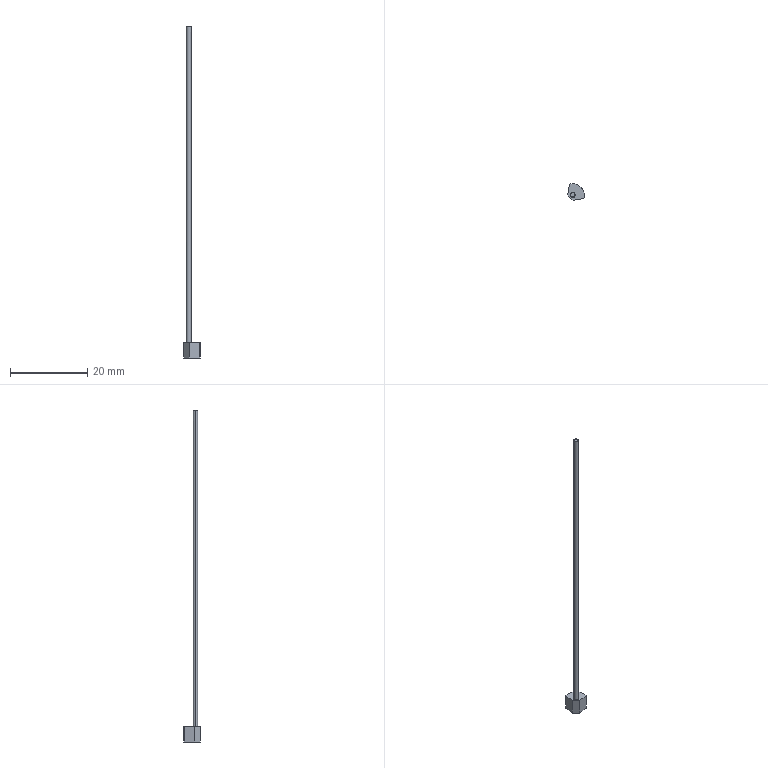Part | Creo | 1 solid | 11 faces | box 4.284 x 4.284 x 86.149 mm | volume 148.672 mm3 | plane 6 | cylinder 3 | cone 2 | commonest cylinder face diameters 1.2 x2 6 x1
STEP:
#1=CARTESIAN_POINT('',(0.,0.,0.));
#2=DIRECTION('',(0.,0.,1.));
#3=DIRECTION('',(1.,0.,0.));
#4=AXIS2_PLACEMENT_3D('',#1,#2,#3);
#5=CARTESIAN_POINT('',(-33.146,-77.496,32.059));
#6=VERTEX_POINT('',#5);
#7=CARTESIAN_POINT('',(-33.746,-76.905,32.05));
#8=VERTEX_POINT('',#7);
#9=CARTESIAN_POINT('',(-33.746,-77.496,32.059));
#10=DIRECTION('',(0.,0.,1.));
#11=DIRECTION('',(1.,0.,0.));
#12=AXIS2_PLACEMENT_3D('',#9,#10,#11);
#13=CIRCLE('',#12,0.6);
#14=EDGE_CURVE('',#6,#8,#13,.T.);
#15=ORIENTED_EDGE('',*,*,#14,.T.);
#16=CARTESIAN_POINT('',(-34.346,-77.496,32.059));
#17=VERTEX_POINT('',#16);
#18=CARTESIAN_POINT('',(-33.746,-77.496,32.059));
#19=DIRECTION('',(0.,0.,1.));
#20=DIRECTION('',(-0.000001887,1.,0.));
#21=AXIS2_PLACEMENT_3D('',#18,#19,#20);
#22=CIRCLE('',#21,0.6);
#23=EDGE_CURVE('',#8,#17,#22,.T.);
#24=ORIENTED_EDGE('',*,*,#23,.T.);
#25=CARTESIAN_POINT('',(-34.346,-77.496,-50.09));
#26=VERTEX_POINT('',#25);
#27=CARTESIAN_POINT('',(-34.346,-77.496,32.059));
#28=DIRECTION('',(0.,0.,-1.));
#29=VECTOR('',#28,82.149);
#30=LINE('',#27,#29);
#31=EDGE_CURVE('',#17,#26,#30,.T.);
#32=ORIENTED_EDGE('',*,*,#31,.T.);
#33=CARTESIAN_POINT('',(-33.146,-77.496,-50.09));
#34=VERTEX_POINT('',#33);
#35=CARTESIAN_POINT('',(-33.746,-77.496,-50.09));
#36=DIRECTION('',(0.,0.,-1.));
#37=DIRECTION('',(-1.,0.,0.));
#38=AXIS2_PLACEMENT_3D('',#35,#36,#37);
#39=CIRCLE('',#38,0.6);
#40=EDGE_CURVE('',#26,#34,#39,.T.);
#41=ORIENTED_EDGE('',*,*,#40,.T.);
#42=CARTESIAN_POINT('',(-33.146,-77.496,32.059));
#43=DIRECTION('',(0.,0.,-1.));
#44=VECTOR('',#43,82.149);
#45=LINE('',#42,#44);
#46=EDGE_CURVE('',#6,#34,#45,.T.);
#47=ORIENTED_EDGE('',*,*,#46,.F.);
#48=EDGE_LOOP('',(#15,#24,#32,#41,#47));
#49=FACE_OUTER_BOUND('',#48,.F.);
#50=CARTESIAN_POINT('',(-33.746,-77.496,32.041));
#51=DIRECTION('',(0.,0.,-1.));
#52=DIRECTION('',(-1.,0.,0.));
#53=AXIS2_PLACEMENT_3D('',#50,#51,#52);
#54=CYLINDRICAL_SURFACE('',#53,0.6);
#55=ADVANCED_FACE('',(#49),#54,.T.);
#56=ORIENTED_EDGE('',*,*,#14,.F.);
#57=CARTESIAN_POINT('',(-33.746,-78.087,32.05));
#58=VERTEX_POINT('',#57);
#59=CARTESIAN_POINT('',(-33.746,-77.496,32.059));
#60=DIRECTION('',(0.,0.,1.));
#61=DIRECTION('',(0.000001887,-1.,0.));
#62=AXIS2_PLACEMENT_3D('',#59,#60,#61);
#63=CIRCLE('',#62,0.6);
#64=EDGE_CURVE('',#58,#6,#63,.T.);
#65=ORIENTED_EDGE('',*,*,#64,.F.);
#66=CARTESIAN_POINT('',(-33.164,-77.496,32.041));
#67=VERTEX_POINT('',#66);
#68=CARTESIAN_POINT('',(-33.746,-78.087,32.05));
#69=CARTESIAN_POINT('',(-33.683,-78.087,32.05));
#70=CARTESIAN_POINT('',(-33.563,-78.054,32.037));
#71=CARTESIAN_POINT('',(-33.398,-77.975,32.042));
#72=CARTESIAN_POINT('',(-33.268,-77.844,32.041));
#73=CARTESIAN_POINT('',(-33.184,-77.679,32.041));
#74=CARTESIAN_POINT('',(-33.164,-77.559,32.041));
#75=B_SPLINE_CURVE_WITH_KNOTS('',3,(#68,#69,#70,#71,#72,#73,#74,#66),.UNSPECIFIED.,.F.,.F.,(4,1,1,1,1,4),(0.,0.2,0.4,0.6,0.8,1.),.UNSPECIFIED.);
#76=EDGE_CURVE('',#58,#67,#75,.T.);
#77=ORIENTED_EDGE('',*,*,#76,.T.);
#78=CARTESIAN_POINT('',(-33.164,-77.496,32.041));
#79=CARTESIAN_POINT('',(-33.164,-77.433,32.041));
#80=CARTESIAN_POINT('',(-33.184,-77.313,32.041));
#81=CARTESIAN_POINT('',(-33.268,-77.148,32.041));
#82=CARTESIAN_POINT('',(-33.398,-77.017,32.042));
#83=CARTESIAN_POINT('',(-33.563,-76.938,32.037));
#84=CARTESIAN_POINT('',(-33.683,-76.905,32.05));
#85=CARTESIAN_POINT('',(-33.746,-76.905,32.05));
#86=B_SPLINE_CURVE_WITH_KNOTS('',3,(#78,#79,#80,#81,#82,#83,#84,#85),.UNSPECIFIED.,.F.,.F.,(4,1,1,1,1,4),(0.,0.2,0.4,0.6,0.8,1.),.UNSPECIFIED.);
#87=EDGE_CURVE('',#67,#8,#86,.T.);
#88=ORIENTED_EDGE('',*,*,#87,.T.);
#89=EDGE_LOOP('',(#56,#65,#77,#88));
#90=FACE_OUTER_BOUND('',#89,.F.);
#91=CARTESIAN_POINT('',(-33.746,-77.496,32.05));
#92=DIRECTION('',(0.,0.,1.));
#93=DIRECTION('',(-1.,0.,0.));
#94=AXIS2_PLACEMENT_3D('',#91,#92,#93);
#95=CONICAL_SURFACE('',#94,0.5907,45.637);
#96=ADVANCED_FACE('',(#90),#95,.F.);
#97=ORIENTED_EDGE('',*,*,#64,.T.);
#98=ORIENTED_EDGE('',*,*,#46,.T.);
#99=CARTESIAN_POINT('',(-33.746,-77.496,-50.09));
#100=DIRECTION('',(0.,0.,-1.));
#101=DIRECTION('',(1.,0.,0.));
#102=AXIS2_PLACEMENT_3D('',#99,#100,#101);
#103=CIRCLE('',#102,0.6);
#104=EDGE_CURVE('',#34,#26,#103,.T.);
#105=ORIENTED_EDGE('',*,*,#104,.T.);
#106=ORIENTED_EDGE('',*,*,#31,.F.);
#107=CARTESIAN_POINT('',(-33.746,-77.496,32.059));
#108=DIRECTION('',(0.,0.,1.));
#109=DIRECTION('',(-1.,0.,0.));
#110=AXIS2_PLACEMENT_3D('',#107,#108,#109);
#111=CIRCLE('',#110,0.6);
#112=EDGE_CURVE('',#17,#58,#111,.T.);
#113=ORIENTED_EDGE('',*,*,#112,.T.);
#114=EDGE_LOOP('',(#97,#98,#105,#106,#113));
#115=FACE_OUTER_BOUND('',#114,.F.);
#116=CARTESIAN_POINT('',(-33.746,-77.496,32.041));
#117=DIRECTION('',(0.,0.,-1.));
#118=DIRECTION('',(-1.,0.,0.));
#119=AXIS2_PLACEMENT_3D('',#116,#117,#118);
#120=CYLINDRICAL_SURFACE('',#119,0.6);
#121=ADVANCED_FACE('',(#115),#120,.T.);
#122=CARTESIAN_POINT('',(-30.873,-78.361,-50.09));
#123=VERTEX_POINT('',#122);
#124=CARTESIAN_POINT('',(-34.611,-74.623,-50.09));
#125=VERTEX_POINT('',#124);
#126=CARTESIAN_POINT('',(-33.746,-77.496,-50.09));
#127=DIRECTION('',(0.,0.,1.));
#128=DIRECTION('',(0.9576,-0.2883,0.));
#129=AXIS2_PLACEMENT_3D('',#126,#127,#128);
#130=CIRCLE('',#129,3.);
#131=EDGE_CURVE('',#123,#125,#130,.T.);
#132=ORIENTED_EDGE('',*,*,#131,.F.);
#133=CARTESIAN_POINT('',(-33.662,-78.78,-50.09));
#134=VERTEX_POINT('',#133);
#135=CARTESIAN_POINT('',(-33.662,-78.78,-50.09));
#136=DIRECTION('',(0.9889,0.1487,0.));
#137=VECTOR('',#136,2.82);
#138=LINE('',#135,#137);
#139=EDGE_CURVE('',#134,#123,#138,.T.);
#140=ORIENTED_EDGE('',*,*,#139,.F.);
#141=CARTESIAN_POINT('',(-35.03,-77.412,-50.09));
#142=VERTEX_POINT('',#141);
#143=CARTESIAN_POINT('',(-35.03,-77.412,-50.09));
#144=DIRECTION('',(0.7071,-0.7071,0.));
#145=VECTOR('',#144,1.935);
#146=LINE('',#143,#145);
#147=EDGE_CURVE('',#142,#134,#146,.T.);
#148=ORIENTED_EDGE('',*,*,#147,.F.);
#149=CARTESIAN_POINT('',(-34.611,-74.623,-50.09));
#150=DIRECTION('',(-0.1487,-0.9889,0.));
#151=VECTOR('',#150,2.82);
#152=LINE('',#149,#151);
#153=EDGE_CURVE('',#125,#142,#152,.T.);
#154=ORIENTED_EDGE('',*,*,#153,.F.);
#155=EDGE_LOOP('',(#132,#140,#148,#154));
#156=FACE_OUTER_BOUND('',#155,.F.);
#157=ORIENTED_EDGE('',*,*,#104,.F.);
#158=ORIENTED_EDGE('',*,*,#40,.F.);
#159=EDGE_LOOP('',(#157,#158));
#160=FACE_BOUND('',#159,.F.);
#161=CARTESIAN_POINT('',(-33.746,-77.496,-50.09));
#162=DIRECTION('',(0.,0.,1.));
#163=DIRECTION('',(1.,0.,0.));
#164=AXIS2_PLACEMENT_3D('',#161,#162,#163);
#165=PLANE('',#164);
#166=ADVANCED_FACE('',(#156,#160),#165,.T.);
#167=CARTESIAN_POINT('',(-30.746,-77.496,-54.09));
#168=VERTEX_POINT('',#167);
#169=CARTESIAN_POINT('',(-30.873,-78.361,-54.09));
#170=VERTEX_POINT('',#169);
#171=CARTESIAN_POINT('',(-33.746,-77.496,-54.09));
#172=DIRECTION('',(0.,0.,-1.));
#173=DIRECTION('',(1.,0.,0.));
#174=AXIS2_PLACEMENT_3D('',#171,#172,#173);
#175=CIRCLE('',#174,3.);
#176=EDGE_CURVE('',#168,#170,#175,.T.);
#177=ORIENTED_EDGE('',*,*,#176,.T.);
#178=CARTESIAN_POINT('',(-30.873,-78.361,-50.09));
#179=DIRECTION('',(0.,0.,-1.));
#180=VECTOR('',#179,4.);
#181=LINE('',#178,#180);
#182=EDGE_CURVE('',#123,#170,#181,.T.);
#183=ORIENTED_EDGE('',*,*,#182,.F.);
#184=ORIENTED_EDGE('',*,*,#131,.T.);
#185=CARTESIAN_POINT('',(-34.611,-74.623,-54.09));
#186=VERTEX_POINT('',#185);
#187=CARTESIAN_POINT('',(-34.611,-74.623,-54.09));
#188=DIRECTION('',(0.,0.,1.));
#189=VECTOR('',#188,4.);
#190=LINE('',#187,#189);
#191=EDGE_CURVE('',#186,#125,#190,.T.);
#192=ORIENTED_EDGE('',*,*,#191,.F.);
#193=CARTESIAN_POINT('',(-33.746,-77.496,-54.09));
#194=DIRECTION('',(0.,0.,-1.));
#195=DIRECTION('',(-0.2883,0.9576,0.));
#196=AXIS2_PLACEMENT_3D('',#193,#194,#195);
#197=CIRCLE('',#196,3.);
#198=EDGE_CURVE('',#186,#168,#197,.T.);
#199=ORIENTED_EDGE('',*,*,#198,.T.);
#200=EDGE_LOOP('',(#177,#183,#184,#192,#199));
#201=FACE_OUTER_BOUND('',#200,.F.);
#202=CARTESIAN_POINT('',(-33.746,-77.496,-44.09));
#203=DIRECTION('',(0.,0.,1.));
#204=DIRECTION('',(1.,0.,0.));
#205=AXIS2_PLACEMENT_3D('',#202,#203,#204);
#206=CYLINDRICAL_SURFACE('',#205,3.);
#207=ADVANCED_FACE('',(#201),#206,.T.);
#208=CARTESIAN_POINT('',(-33.662,-78.78,-54.09));
#209=VERTEX_POINT('',#208);
#210=CARTESIAN_POINT('',(-35.03,-77.412,-54.09));
#211=VERTEX_POINT('',#210);
#212=CARTESIAN_POINT('',(-33.662,-78.78,-54.09));
#213=DIRECTION('',(-0.7071,0.7071,0.));
#214=VECTOR('',#213,1.935);
#215=LINE('',#212,#214);
#216=EDGE_CURVE('',#209,#211,#215,.T.);
#217=ORIENTED_EDGE('',*,*,#216,.F.);
#218=CARTESIAN_POINT('',(-30.873,-78.361,-54.09));
#219=DIRECTION('',(-0.9889,-0.1487,0.));
#220=VECTOR('',#219,2.82);
#221=LINE('',#218,#220);
#222=EDGE_CURVE('',#170,#209,#221,.T.);
#223=ORIENTED_EDGE('',*,*,#222,.F.);
#224=ORIENTED_EDGE('',*,*,#176,.F.);
#225=ORIENTED_EDGE('',*,*,#198,.F.);
#226=CARTESIAN_POINT('',(-35.03,-77.412,-54.09));
#227=DIRECTION('',(0.1487,0.9889,0.));
#228=VECTOR('',#227,2.82);
#229=LINE('',#226,#228);
#230=EDGE_CURVE('',#211,#186,#229,.T.);
#231=ORIENTED_EDGE('',*,*,#230,.F.);
#232=EDGE_LOOP('',(#217,#223,#224,#225,#231));
#233=FACE_OUTER_BOUND('',#232,.F.);
#234=CARTESIAN_POINT('',(0.,0.,-54.09));
#235=DIRECTION('',(0.,0.,-1.));
#236=DIRECTION('',(-1.,0.,0.));
#237=AXIS2_PLACEMENT_3D('',#234,#235,#236);
#238=PLANE('',#237);
#239=ADVANCED_FACE('',(#233),#238,.T.);
#240=ORIENTED_EDGE('',*,*,#147,.T.);
#241=CARTESIAN_POINT('',(-33.662,-78.78,-50.09));
#242=DIRECTION('',(0.,0.,-1.));
#243=VECTOR('',#242,4.);
#244=LINE('',#241,#243);
#245=EDGE_CURVE('',#134,#209,#244,.T.);
#246=ORIENTED_EDGE('',*,*,#245,.T.);
#247=ORIENTED_EDGE('',*,*,#216,.T.);
#248=CARTESIAN_POINT('',(-35.03,-77.412,-54.09));
#249=DIRECTION('',(0.,0.,1.));
#250=VECTOR('',#249,4.);
#251=LINE('',#248,#250);
#252=EDGE_CURVE('',#211,#142,#251,.T.);
#253=ORIENTED_EDGE('',*,*,#252,.T.);
#254=EDGE_LOOP('',(#240,#246,#247,#253));
#255=FACE_OUTER_BOUND('',#254,.F.);
#256=CARTESIAN_POINT('',(-34.346,-78.096,-54.09));
#257=DIRECTION('',(0.7071,0.7071,0.));
#258=DIRECTION('',(-0.7071,0.7071,0.));
#259=AXIS2_PLACEMENT_3D('',#256,#257,#258);
#260=PLANE('',#259);
#261=ADVANCED_FACE('',(#255),#260,.F.);
#262=ORIENTED_EDGE('',*,*,#222,.T.);
#263=ORIENTED_EDGE('',*,*,#245,.F.);
#264=ORIENTED_EDGE('',*,*,#139,.T.);
#265=ORIENTED_EDGE('',*,*,#182,.T.);
#266=EDGE_LOOP('',(#262,#263,#264,#265));
#267=FACE_OUTER_BOUND('',#266,.F.);
#268=CARTESIAN_POINT('',(-33.296,-78.725,-44.09));
#269=DIRECTION('',(-0.1487,0.9889,0.));
#270=DIRECTION('',(0.,0.,1.));
#271=AXIS2_PLACEMENT_3D('',#268,#269,#270);
#272=PLANE('',#271);
#273=ADVANCED_FACE('',(#267),#272,.F.);
#274=ORIENTED_EDGE('',*,*,#153,.T.);
#275=ORIENTED_EDGE('',*,*,#252,.F.);
#276=ORIENTED_EDGE('',*,*,#230,.T.);
#277=ORIENTED_EDGE('',*,*,#191,.T.);
#278=EDGE_LOOP('',(#274,#275,#276,#277));
#279=FACE_OUTER_BOUND('',#278,.F.);
#280=CARTESIAN_POINT('',(-34.975,-77.047,-44.09));
#281=DIRECTION('',(-0.9889,0.1487,0.));
#282=DIRECTION('',(0.,0.,1.));
#283=AXIS2_PLACEMENT_3D('',#280,#281,#282);
#284=PLANE('',#283);
#285=ADVANCED_FACE('',(#279),#284,.T.);
#286=ORIENTED_EDGE('',*,*,#23,.F.);
#287=CARTESIAN_POINT('',(-33.817,-76.905,32.05));
#288=CARTESIAN_POINT('',(-33.949,-76.943,32.037));
#289=CARTESIAN_POINT('',(-34.128,-77.041,32.042));
#290=CARTESIAN_POINT('',(-34.258,-77.198,32.041));
#291=CARTESIAN_POINT('',(-34.33,-77.391,32.041));
#292=CARTESIAN_POINT('',(-34.331,-77.597,32.041));
#293=CARTESIAN_POINT('',(-34.261,-77.79,32.041));
#294=CARTESIAN_POINT('',(-34.131,-77.949,32.042));
#295=CARTESIAN_POINT('',(-33.949,-78.049,32.037));
#296=CARTESIAN_POINT('',(-33.817,-78.087,32.05));
#297=B_SPLINE_CURVE_WITH_KNOTS('',3,(#7,#287,#288,#289,#290,#291,#292,#293,#294,#295,#296,#57),.UNSPECIFIED.,.F.,.F.,(4,1,1,1,1,1,1,1,1,4),(0.,0.1111,0.2222,0.3333,0.4444,0.5556,0.6667,0.7778,0.8889,1.),.UNSPECIFIED.);
#298=EDGE_CURVE('',#8,#58,#297,.T.);
#299=ORIENTED_EDGE('',*,*,#298,.T.);
#300=ORIENTED_EDGE('',*,*,#112,.F.);
#301=EDGE_LOOP('',(#286,#299,#300));
#302=FACE_OUTER_BOUND('',#301,.F.);
#303=CARTESIAN_POINT('',(-33.746,-77.496,32.05));
#304=DIRECTION('',(0.,0.,1.));
#305=DIRECTION('',(-1.,0.,0.));
#306=AXIS2_PLACEMENT_3D('',#303,#304,#305);
#307=CONICAL_SURFACE('',#306,0.5907,45.637);
#308=ADVANCED_FACE('',(#302),#307,.F.);
#309=ORIENTED_EDGE('',*,*,#298,.F.);
#310=ORIENTED_EDGE('',*,*,#87,.F.);
#311=ORIENTED_EDGE('',*,*,#76,.F.);
#312=EDGE_LOOP('',(#309,#310,#311));
#313=FACE_OUTER_BOUND('',#312,.F.);
#314=CARTESIAN_POINT('',(-0.07825,-88.35,32.041));
#315=DIRECTION('',(0.,0.,-1.));
#316=DIRECTION('',(0.,-1.,0.));
#317=AXIS2_PLACEMENT_3D('',#314,#315,#316);
#318=PLANE('',#317);
#319=ADVANCED_FACE('',(#313),#318,.F.);
#320=CLOSED_SHELL('',(#55,#96,#121,#166,#207,#239,#261,#273,#285,#308,#319));
#321=MANIFOLD_SOLID_BREP('',#320);
#322=(LENGTH_UNIT()NAMED_UNIT(*)SI_UNIT(.MILLI.,.METRE.));
#323=UNCERTAINTY_MEASURE_WITH_UNIT(LENGTH_MEASURE(0.01298),#322,'','');
#324=(NAMED_UNIT(*)PLANE_ANGLE_UNIT()SI_UNIT($,.RADIAN.));
#325=PLANE_ANGLE_MEASURE_WITH_UNIT(PLANE_ANGLE_MEASURE(0.01745),#324);
#326=(CONVERSION_BASED_UNIT('DEGREE',#325)NAMED_UNIT(*)PLANE_ANGLE_UNIT());
#327=(NAMED_UNIT(*)SI_UNIT($,.STERADIAN.)SOLID_ANGLE_UNIT());
#328=(GEOMETRIC_REPRESENTATION_CONTEXT(3)GLOBAL_UNCERTAINTY_ASSIGNED_CONTEXT((#323))GLOBAL_UNIT_ASSIGNED_CONTEXT((#322,#326,#327))REPRESENTATION_CONTEXT('',''));
#329=ADVANCED_BREP_SHAPE_REPRESENTATION('',(#4,#321),#328);